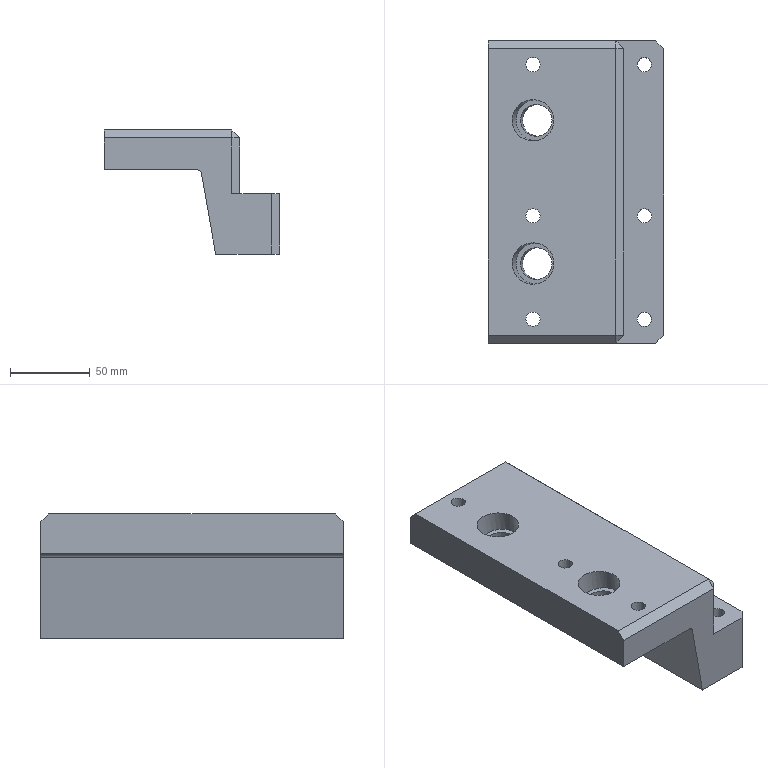Part | STEP file | P011002S002-012 | 1 solid | 44 faces | box 110 x 190 x 78 mm | volume 738525 mm3 | plane 27 | cylinder 17 | commonest cylinder face diameters 9 x6 14 x6 20 x2 26 x2 6 x1